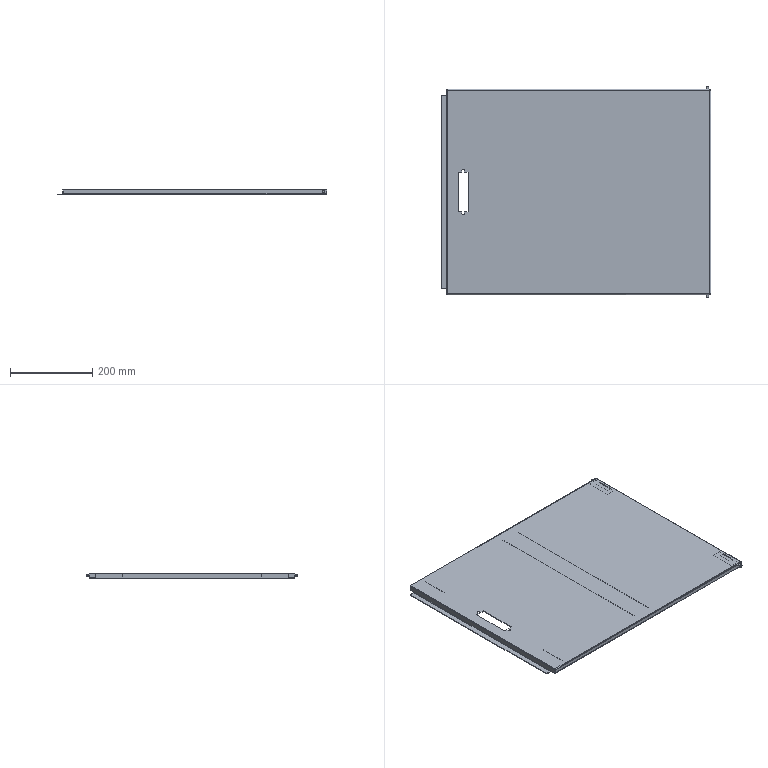Part | SolidWorks | features BaseBody 6 | 6 solids | 198 faces | box 655.5 x 513 x 14.5 mm | volume 627122 mm3 | plane 106 | cylinder 60 | spline 28 | torus 4 | commonest cylinder face diameters 5 x16 1.473 x14 4.473 x14 9 x12 6 x2 10 x2